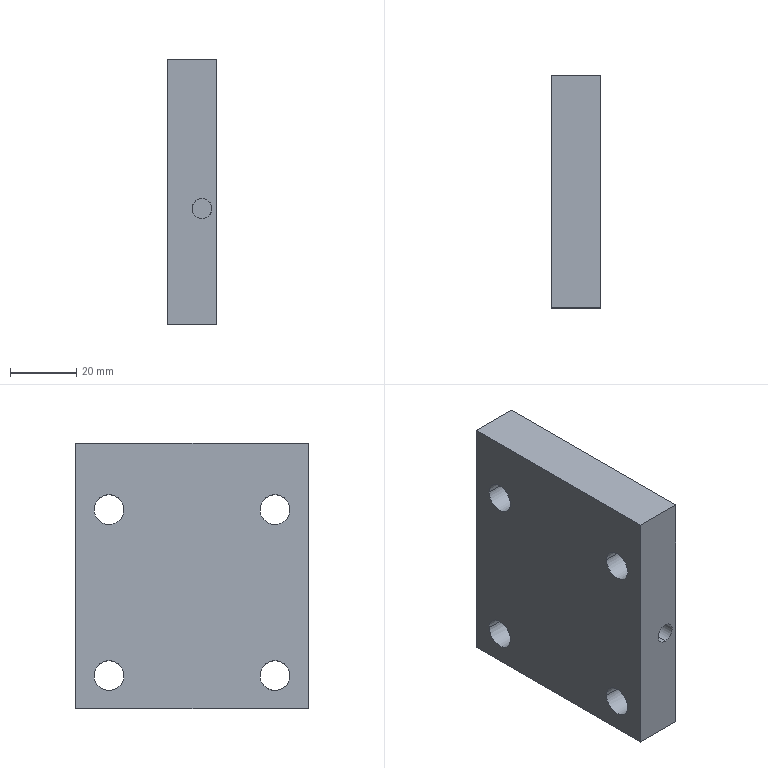Part | STEP file | Positioning_id1838_x_t | 1 solid | 21 faces | box 15 x 70 x 80 mm | volume 79602 mm3 | cylinder 14 | plane 7 | commonest cylinder face diameters 9 x8 6 x6